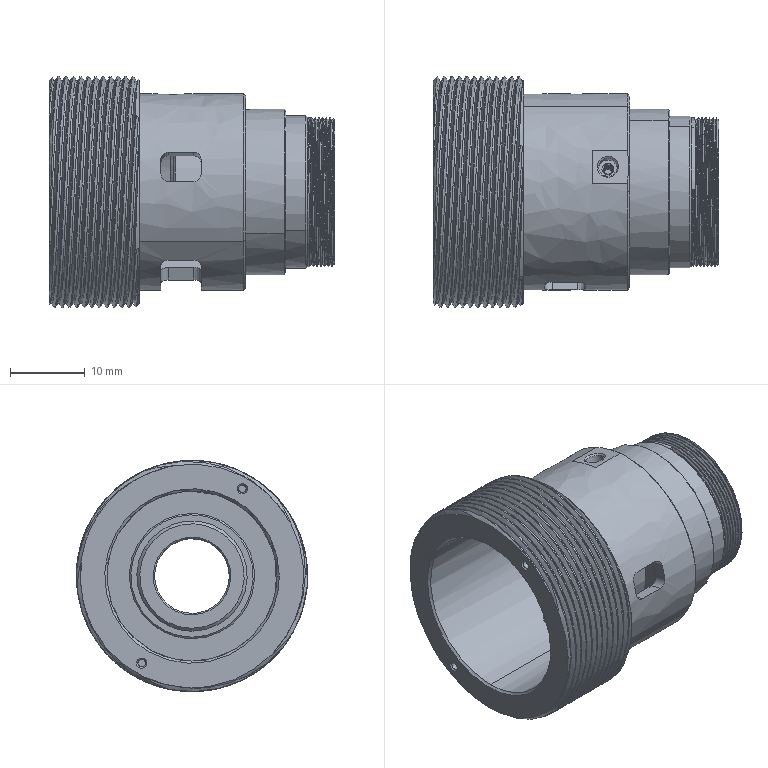Part | SolidWorks | features BaseBody 1 | 1 solid | 234 faces | box 38.251 x 31 x 31 mm | volume 8383 mm3 | cylinder 88 | spline 66 | cone 44 | plane 36 | commonest cylinder face diameters 31 x20 20 x16 1.2 x14 2 x12 10 x3 12.6 x3